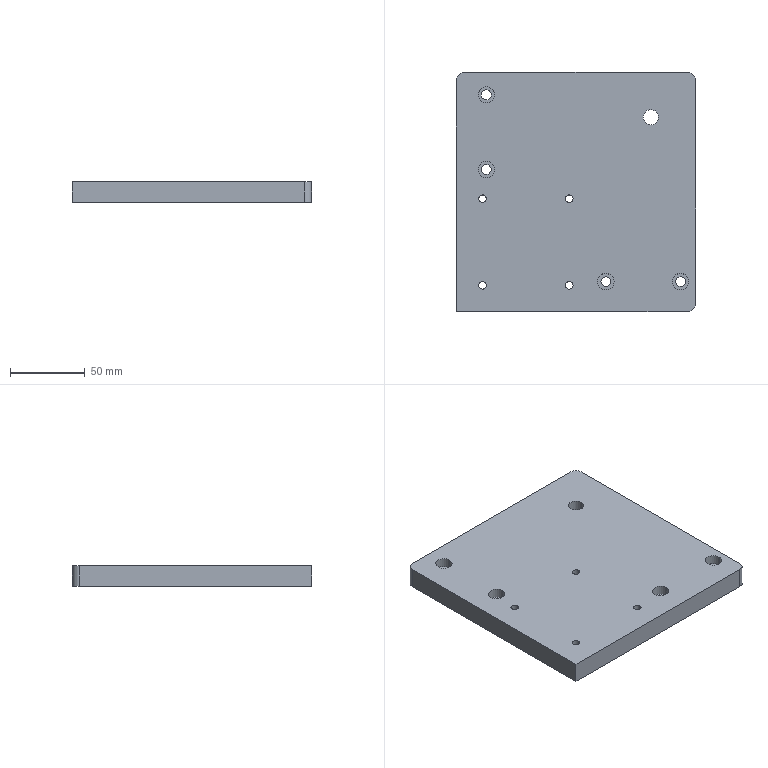Part | STEP file | HJ60 Fuma caster mounting plate -A0 | 1 solid | 39 faces | box 160 x 160 x 14 mm | volume 352458 mm3 | cylinder 29 | plane 10 | commonest cylinder face diameters 5 x8 6.6 x8 11 x8 10 x3 10.2 x2
STEP:
#1=CARTESIAN_POINT('',(-65.,-62.5,0.));
#2=VERTEX_POINT('',#1);
#3=CARTESIAN_POINT('',(-60.,-62.5,0.));
#4=VERTEX_POINT('',#3);
#5=CARTESIAN_POINT('',(-62.5,-62.5,0.));
#6=DIRECTION('',(0.,0.,1.));
#7=DIRECTION('',(1.,0.,0.));
#8=AXIS2_PLACEMENT_3D('',#5,#6,#7);
#9=CIRCLE('',#8,2.5);
#10=EDGE_CURVE('',#2,#4,#9,.T.);
#11=ORIENTED_EDGE('',*,*,#10,.F.);
#12=CARTESIAN_POINT('',(-65.,-62.5,14.));
#13=VERTEX_POINT('',#12);
#14=CARTESIAN_POINT('',(-65.,-62.5,14.));
#15=DIRECTION('',(0.,0.,1.));
#16=VECTOR('',#15,1000.);
#17=LINE('',#14,#16);
#18=EDGE_CURVE('',#2,#13,#17,.T.);
#19=ORIENTED_EDGE('',*,*,#18,.T.);
#20=CARTESIAN_POINT('',(-60.,-62.5,14.));
#21=VERTEX_POINT('',#20);
#22=CARTESIAN_POINT('',(-62.5,-62.5,14.));
#23=DIRECTION('',(0.,0.,-1.));
#24=DIRECTION('',(1.,0.,0.));
#25=AXIS2_PLACEMENT_3D('',#22,#23,#24);
#26=CIRCLE('',#25,2.5);
#27=EDGE_CURVE('',#21,#13,#26,.T.);
#28=ORIENTED_EDGE('',*,*,#27,.F.);
#29=CARTESIAN_POINT('',(-60.,-62.5,14.));
#30=DIRECTION('',(0.,0.,1.));
#31=VECTOR('',#30,1000.);
#32=LINE('',#29,#31);
#33=EDGE_CURVE('',#4,#21,#32,.T.);
#34=ORIENTED_EDGE('',*,*,#33,.F.);
#35=EDGE_LOOP('',(#11,#19,#28,#34));
#36=FACE_OUTER_BOUND('',#35,.T.);
#37=CARTESIAN_POINT('',(-62.5,-62.5,14.));
#38=DIRECTION('',(0.,0.,1.));
#39=DIRECTION('',(1.,0.,0.));
#40=AXIS2_PLACEMENT_3D('',#37,#38,#39);
#41=CYLINDRICAL_SURFACE('',#40,2.5);
#42=ADVANCED_FACE('',(#36),#41,.F.);
#43=CARTESIAN_POINT('',(-7.,-62.5,0.));
#44=VERTEX_POINT('',#43);
#45=CARTESIAN_POINT('',(-2.,-62.5,0.));
#46=VERTEX_POINT('',#45);
#47=CARTESIAN_POINT('',(-4.5,-62.5,0.));
#48=DIRECTION('',(0.,0.,1.));
#49=DIRECTION('',(1.,0.,0.));
#50=AXIS2_PLACEMENT_3D('',#47,#48,#49);
#51=CIRCLE('',#50,2.5);
#52=EDGE_CURVE('',#44,#46,#51,.T.);
#53=ORIENTED_EDGE('',*,*,#52,.F.);
#54=CARTESIAN_POINT('',(-7.,-62.5,14.));
#55=VERTEX_POINT('',#54);
#56=CARTESIAN_POINT('',(-7.,-62.5,14.));
#57=DIRECTION('',(0.,0.,1.));
#58=VECTOR('',#57,1000.);
#59=LINE('',#56,#58);
#60=EDGE_CURVE('',#44,#55,#59,.T.);
#61=ORIENTED_EDGE('',*,*,#60,.T.);
#62=CARTESIAN_POINT('',(-2.,-62.5,14.));
#63=VERTEX_POINT('',#62);
#64=CARTESIAN_POINT('',(-4.5,-62.5,14.));
#65=DIRECTION('',(0.,0.,-1.));
#66=DIRECTION('',(1.,0.,0.));
#67=AXIS2_PLACEMENT_3D('',#64,#65,#66);
#68=CIRCLE('',#67,2.5);
#69=EDGE_CURVE('',#63,#55,#68,.T.);
#70=ORIENTED_EDGE('',*,*,#69,.F.);
#71=CARTESIAN_POINT('',(-2.,-62.5,14.));
#72=DIRECTION('',(0.,0.,1.));
#73=VECTOR('',#72,1000.);
#74=LINE('',#71,#73);
#75=EDGE_CURVE('',#46,#63,#74,.T.);
#76=ORIENTED_EDGE('',*,*,#75,.F.);
#77=EDGE_LOOP('',(#53,#61,#70,#76));
#78=FACE_OUTER_BOUND('',#77,.T.);
#79=CARTESIAN_POINT('',(-4.5,-62.5,14.));
#80=DIRECTION('',(0.,0.,1.));
#81=DIRECTION('',(1.,0.,0.));
#82=AXIS2_PLACEMENT_3D('',#79,#80,#81);
#83=CYLINDRICAL_SURFACE('',#82,2.5);
#84=ADVANCED_FACE('',(#78),#83,.F.);
#85=CARTESIAN_POINT('',(-7.,-4.5,0.));
#86=VERTEX_POINT('',#85);
#87=CARTESIAN_POINT('',(-2.,-4.5,0.));
#88=VERTEX_POINT('',#87);
#89=CARTESIAN_POINT('',(-4.5,-4.5,0.));
#90=DIRECTION('',(0.,0.,1.));
#91=DIRECTION('',(1.,0.,0.));
#92=AXIS2_PLACEMENT_3D('',#89,#90,#91);
#93=CIRCLE('',#92,2.5);
#94=EDGE_CURVE('',#86,#88,#93,.T.);
#95=ORIENTED_EDGE('',*,*,#94,.F.);
#96=CARTESIAN_POINT('',(-7.,-4.5,14.));
#97=VERTEX_POINT('',#96);
#98=CARTESIAN_POINT('',(-7.,-4.5,14.));
#99=DIRECTION('',(0.,0.,1.));
#100=VECTOR('',#99,1000.);
#101=LINE('',#98,#100);
#102=EDGE_CURVE('',#86,#97,#101,.T.);
#103=ORIENTED_EDGE('',*,*,#102,.T.);
#104=CARTESIAN_POINT('',(-2.,-4.5,14.));
#105=VERTEX_POINT('',#104);
#106=CARTESIAN_POINT('',(-4.5,-4.5,14.));
#107=DIRECTION('',(0.,0.,-1.));
#108=DIRECTION('',(1.,0.,0.));
#109=AXIS2_PLACEMENT_3D('',#106,#107,#108);
#110=CIRCLE('',#109,2.5);
#111=EDGE_CURVE('',#105,#97,#110,.T.);
#112=ORIENTED_EDGE('',*,*,#111,.F.);
#113=CARTESIAN_POINT('',(-2.,-4.5,14.));
#114=DIRECTION('',(0.,0.,1.));
#115=VECTOR('',#114,1000.);
#116=LINE('',#113,#115);
#117=EDGE_CURVE('',#88,#105,#116,.T.);
#118=ORIENTED_EDGE('',*,*,#117,.F.);
#119=EDGE_LOOP('',(#95,#103,#112,#118));
#120=FACE_OUTER_BOUND('',#119,.T.);
#121=CARTESIAN_POINT('',(-4.5,-4.5,14.));
#122=DIRECTION('',(0.,0.,1.));
#123=DIRECTION('',(1.,0.,0.));
#124=AXIS2_PLACEMENT_3D('',#121,#122,#123);
#125=CYLINDRICAL_SURFACE('',#124,2.5);
#126=ADVANCED_FACE('',(#120),#125,.F.);
#127=CARTESIAN_POINT('',(-65.,-4.5,0.));
#128=VERTEX_POINT('',#127);
#129=CARTESIAN_POINT('',(-60.,-4.5,0.));
#130=VERTEX_POINT('',#129);
#131=CARTESIAN_POINT('',(-62.5,-4.5,0.));
#132=DIRECTION('',(0.,0.,1.));
#133=DIRECTION('',(1.,0.,0.));
#134=AXIS2_PLACEMENT_3D('',#131,#132,#133);
#135=CIRCLE('',#134,2.5);
#136=EDGE_CURVE('',#128,#130,#135,.T.);
#137=ORIENTED_EDGE('',*,*,#136,.F.);
#138=CARTESIAN_POINT('',(-65.,-4.5,14.));
#139=VERTEX_POINT('',#138);
#140=CARTESIAN_POINT('',(-65.,-4.5,14.));
#141=DIRECTION('',(0.,0.,1.));
#142=VECTOR('',#141,1000.);
#143=LINE('',#140,#142);
#144=EDGE_CURVE('',#128,#139,#143,.T.);
#145=ORIENTED_EDGE('',*,*,#144,.T.);
#146=CARTESIAN_POINT('',(-60.,-4.5,14.));
#147=VERTEX_POINT('',#146);
#148=CARTESIAN_POINT('',(-62.5,-4.5,14.));
#149=DIRECTION('',(0.,0.,-1.));
#150=DIRECTION('',(1.,0.,0.));
#151=AXIS2_PLACEMENT_3D('',#148,#149,#150);
#152=CIRCLE('',#151,2.5);
#153=EDGE_CURVE('',#147,#139,#152,.T.);
#154=ORIENTED_EDGE('',*,*,#153,.F.);
#155=CARTESIAN_POINT('',(-60.,-4.5,14.));
#156=DIRECTION('',(0.,0.,1.));
#157=VECTOR('',#156,1000.);
#158=LINE('',#155,#157);
#159=EDGE_CURVE('',#130,#147,#158,.T.);
#160=ORIENTED_EDGE('',*,*,#159,.F.);
#161=EDGE_LOOP('',(#137,#145,#154,#160));
#162=FACE_OUTER_BOUND('',#161,.T.);
#163=CARTESIAN_POINT('',(-62.5,-4.5,14.));
#164=DIRECTION('',(0.,0.,1.));
#165=DIRECTION('',(1.,0.,0.));
#166=AXIS2_PLACEMENT_3D('',#163,#164,#165);
#167=CYLINDRICAL_SURFACE('',#166,2.5);
#168=ADVANCED_FACE('',(#162),#167,.F.);
#169=CARTESIAN_POINT('',(44.9,50.,0.));
#170=VERTEX_POINT('',#169);
#171=CARTESIAN_POINT('',(55.1,50.,0.));
#172=VERTEX_POINT('',#171);
#173=CARTESIAN_POINT('',(50.,50.,0.));
#174=DIRECTION('',(0.,0.,1.));
#175=DIRECTION('',(1.,0.,0.));
#176=AXIS2_PLACEMENT_3D('',#173,#174,#175);
#177=CIRCLE('',#176,5.1);
#178=EDGE_CURVE('',#170,#172,#177,.T.);
#179=ORIENTED_EDGE('',*,*,#178,.F.);
#180=CARTESIAN_POINT('',(44.9,50.,14.));
#181=VERTEX_POINT('',#180);
#182=CARTESIAN_POINT('',(44.9,50.,14.));
#183=DIRECTION('',(0.,0.,1.));
#184=VECTOR('',#183,1000.);
#185=LINE('',#182,#184);
#186=EDGE_CURVE('',#170,#181,#185,.T.);
#187=ORIENTED_EDGE('',*,*,#186,.T.);
#188=CARTESIAN_POINT('',(55.1,50.,14.));
#189=VERTEX_POINT('',#188);
#190=CARTESIAN_POINT('',(50.,50.,14.));
#191=DIRECTION('',(0.,0.,-1.));
#192=DIRECTION('',(1.,0.,0.));
#193=AXIS2_PLACEMENT_3D('',#190,#191,#192);
#194=CIRCLE('',#193,5.1);
#195=EDGE_CURVE('',#189,#181,#194,.T.);
#196=ORIENTED_EDGE('',*,*,#195,.F.);
#197=CARTESIAN_POINT('',(55.1,50.,14.));
#198=DIRECTION('',(0.,0.,1.));
#199=VECTOR('',#198,1000.);
#200=LINE('',#197,#199);
#201=EDGE_CURVE('',#172,#189,#200,.T.);
#202=ORIENTED_EDGE('',*,*,#201,.F.);
#203=EDGE_LOOP('',(#179,#187,#196,#202));
#204=FACE_OUTER_BOUND('',#203,.T.);
#205=CARTESIAN_POINT('',(50.,50.,14.));
#206=DIRECTION('',(0.,0.,1.));
#207=DIRECTION('',(1.,0.,0.));
#208=AXIS2_PLACEMENT_3D('',#205,#206,#207);
#209=CYLINDRICAL_SURFACE('',#208,5.1);
#210=ADVANCED_FACE('',(#204),#209,.F.);
#211=CARTESIAN_POINT('',(16.7,-60.,0.));
#212=VERTEX_POINT('',#211);
#213=CARTESIAN_POINT('',(23.3,-60.,0.));
#214=VERTEX_POINT('',#213);
#215=CARTESIAN_POINT('',(20.,-60.,0.));
#216=DIRECTION('',(0.,0.,1.));
#217=DIRECTION('',(1.,0.,0.));
#218=AXIS2_PLACEMENT_3D('',#215,#216,#217);
#219=CIRCLE('',#218,3.3);
#220=EDGE_CURVE('',#212,#214,#219,.T.);
#221=ORIENTED_EDGE('',*,*,#220,.F.);
#222=CARTESIAN_POINT('',(16.7,-60.,7.6));
#223=VERTEX_POINT('',#222);
#224=CARTESIAN_POINT('',(16.7,-60.,14.));
#225=DIRECTION('',(0.,0.,1.));
#226=VECTOR('',#225,1000.);
#227=LINE('',#224,#226);
#228=EDGE_CURVE('',#212,#223,#227,.T.);
#229=ORIENTED_EDGE('',*,*,#228,.T.);
#230=CARTESIAN_POINT('',(23.3,-60.,7.6));
#231=VERTEX_POINT('',#230);
#232=CARTESIAN_POINT('',(20.,-60.,7.6));
#233=DIRECTION('',(0.,0.,-1.));
#234=DIRECTION('',(1.,0.,0.));
#235=AXIS2_PLACEMENT_3D('',#232,#233,#234);
#236=CIRCLE('',#235,3.3);
#237=EDGE_CURVE('',#231,#223,#236,.T.);
#238=ORIENTED_EDGE('',*,*,#237,.F.);
#239=CARTESIAN_POINT('',(23.3,-60.,14.));
#240=DIRECTION('',(0.,0.,1.));
#241=VECTOR('',#240,1000.);
#242=LINE('',#239,#241);
#243=EDGE_CURVE('',#214,#231,#242,.T.);
#244=ORIENTED_EDGE('',*,*,#243,.F.);
#245=EDGE_LOOP('',(#221,#229,#238,#244));
#246=FACE_OUTER_BOUND('',#245,.T.);
#247=CARTESIAN_POINT('',(20.,-60.,14.));
#248=DIRECTION('',(0.,0.,1.));
#249=DIRECTION('',(1.,0.,0.));
#250=AXIS2_PLACEMENT_3D('',#247,#248,#249);
#251=CYLINDRICAL_SURFACE('',#250,3.3);
#252=ADVANCED_FACE('',(#246),#251,.F.);
#253=CARTESIAN_POINT('',(66.7,-60.,0.));
#254=VERTEX_POINT('',#253);
#255=CARTESIAN_POINT('',(73.3,-60.,0.));
#256=VERTEX_POINT('',#255);
#257=CARTESIAN_POINT('',(70.,-60.,0.));
#258=DIRECTION('',(0.,0.,1.));
#259=DIRECTION('',(1.,0.,0.));
#260=AXIS2_PLACEMENT_3D('',#257,#258,#259);
#261=CIRCLE('',#260,3.3);
#262=EDGE_CURVE('',#254,#256,#261,.T.);
#263=ORIENTED_EDGE('',*,*,#262,.F.);
#264=CARTESIAN_POINT('',(66.7,-60.,7.6));
#265=VERTEX_POINT('',#264);
#266=CARTESIAN_POINT('',(66.7,-60.,14.));
#267=DIRECTION('',(0.,0.,1.));
#268=VECTOR('',#267,1000.);
#269=LINE('',#266,#268);
#270=EDGE_CURVE('',#254,#265,#269,.T.);
#271=ORIENTED_EDGE('',*,*,#270,.T.);
#272=CARTESIAN_POINT('',(73.3,-60.,7.6));
#273=VERTEX_POINT('',#272);
#274=CARTESIAN_POINT('',(70.,-60.,7.6));
#275=DIRECTION('',(0.,0.,-1.));
#276=DIRECTION('',(1.,0.,0.));
#277=AXIS2_PLACEMENT_3D('',#274,#275,#276);
#278=CIRCLE('',#277,3.3);
#279=EDGE_CURVE('',#273,#265,#278,.T.);
#280=ORIENTED_EDGE('',*,*,#279,.F.);
#281=CARTESIAN_POINT('',(73.3,-60.,14.));
#282=DIRECTION('',(0.,0.,1.));
#283=VECTOR('',#282,1000.);
#284=LINE('',#281,#283);
#285=EDGE_CURVE('',#256,#273,#284,.T.);
#286=ORIENTED_EDGE('',*,*,#285,.F.);
#287=EDGE_LOOP('',(#263,#271,#280,#286));
#288=FACE_OUTER_BOUND('',#287,.T.);
#289=CARTESIAN_POINT('',(70.,-60.,14.));
#290=DIRECTION('',(0.,0.,1.));
#291=DIRECTION('',(1.,0.,0.));
#292=AXIS2_PLACEMENT_3D('',#289,#290,#291);
#293=CYLINDRICAL_SURFACE('',#292,3.3);
#294=ADVANCED_FACE('',(#288),#293,.F.);
#295=CARTESIAN_POINT('',(-63.3,15.,0.));
#296=VERTEX_POINT('',#295);
#297=CARTESIAN_POINT('',(-56.7,15.,0.));
#298=VERTEX_POINT('',#297);
#299=CARTESIAN_POINT('',(-60.,15.,0.));
#300=DIRECTION('',(0.,0.,1.));
#301=DIRECTION('',(1.,0.,0.));
#302=AXIS2_PLACEMENT_3D('',#299,#300,#301);
#303=CIRCLE('',#302,3.3);
#304=EDGE_CURVE('',#296,#298,#303,.T.);
#305=ORIENTED_EDGE('',*,*,#304,.F.);
#306=CARTESIAN_POINT('',(-63.3,15.,7.6));
#307=VERTEX_POINT('',#306);
#308=CARTESIAN_POINT('',(-63.3,15.,14.));
#309=DIRECTION('',(0.,0.,1.));
#310=VECTOR('',#309,1000.);
#311=LINE('',#308,#310);
#312=EDGE_CURVE('',#296,#307,#311,.T.);
#313=ORIENTED_EDGE('',*,*,#312,.T.);
#314=CARTESIAN_POINT('',(-56.7,15.,7.6));
#315=VERTEX_POINT('',#314);
#316=CARTESIAN_POINT('',(-60.,15.,7.6));
#317=DIRECTION('',(0.,0.,-1.));
#318=DIRECTION('',(1.,0.,0.));
#319=AXIS2_PLACEMENT_3D('',#316,#317,#318);
#320=CIRCLE('',#319,3.3);
#321=EDGE_CURVE('',#315,#307,#320,.T.);
#322=ORIENTED_EDGE('',*,*,#321,.F.);
#323=CARTESIAN_POINT('',(-56.7,15.,14.));
#324=DIRECTION('',(0.,0.,1.));
#325=VECTOR('',#324,1000.);
#326=LINE('',#323,#325);
#327=EDGE_CURVE('',#298,#315,#326,.T.);
#328=ORIENTED_EDGE('',*,*,#327,.F.);
#329=EDGE_LOOP('',(#305,#313,#322,#328));
#330=FACE_OUTER_BOUND('',#329,.T.);
#331=CARTESIAN_POINT('',(-60.,15.,14.));
#332=DIRECTION('',(0.,0.,1.));
#333=DIRECTION('',(1.,0.,0.));
#334=AXIS2_PLACEMENT_3D('',#331,#332,#333);
#335=CYLINDRICAL_SURFACE('',#334,3.3);
#336=ADVANCED_FACE('',(#330),#335,.F.);
#337=CARTESIAN_POINT('',(-63.3,65.,0.));
#338=VERTEX_POINT('',#337);
#339=CARTESIAN_POINT('',(-56.7,65.,0.));
#340=VERTEX_POINT('',#339);
#341=CARTESIAN_POINT('',(-60.,65.,0.));
#342=DIRECTION('',(0.,0.,1.));
#343=DIRECTION('',(1.,0.,0.));
#344=AXIS2_PLACEMENT_3D('',#341,#342,#343);
#345=CIRCLE('',#344,3.3);
#346=EDGE_CURVE('',#338,#340,#345,.T.);
#347=ORIENTED_EDGE('',*,*,#346,.F.);
#348=CARTESIAN_POINT('',(-63.3,65.,7.6));
#349=VERTEX_POINT('',#348);
#350=CARTESIAN_POINT('',(-63.3,65.,14.));
#351=DIRECTION('',(0.,0.,1.));
#352=VECTOR('',#351,1000.);
#353=LINE('',#350,#352);
#354=EDGE_CURVE('',#338,#349,#353,.T.);
#355=ORIENTED_EDGE('',*,*,#354,.T.);
#356=CARTESIAN_POINT('',(-56.7,65.,7.6));
#357=VERTEX_POINT('',#356);
#358=CARTESIAN_POINT('',(-60.,65.,7.6));
#359=DIRECTION('',(0.,0.,-1.));
#360=DIRECTION('',(1.,0.,0.));
#361=AXIS2_PLACEMENT_3D('',#358,#359,#360);
#362=CIRCLE('',#361,3.3);
#363=EDGE_CURVE('',#357,#349,#362,.T.);
#364=ORIENTED_EDGE('',*,*,#363,.F.);
#365=CARTESIAN_POINT('',(-56.7,65.,14.));
#366=DIRECTION('',(0.,0.,1.));
#367=VECTOR('',#366,1000.);
#368=LINE('',#365,#367);
#369=EDGE_CURVE('',#340,#357,#368,.T.);
#370=ORIENTED_EDGE('',*,*,#369,.F.);
#371=EDGE_LOOP('',(#347,#355,#364,#370));
#372=FACE_OUTER_BOUND('',#371,.T.);
#373=CARTESIAN_POINT('',(-60.,65.,14.));
#374=DIRECTION('',(0.,0.,1.));
#375=DIRECTION('',(1.,0.,0.));
#376=AXIS2_PLACEMENT_3D('',#373,#374,#375);
#377=CYLINDRICAL_SURFACE('',#376,3.3);
#378=ADVANCED_FACE('',(#372),#377,.F.);
#379=CARTESIAN_POINT('',(25.5,-60.,7.6));
#380=VERTEX_POINT('',#379);
#381=CARTESIAN_POINT('',(14.5,-60.,7.6));
#382=VERTEX_POINT('',#381);
#383=CARTESIAN_POINT('',(20.,-60.,7.6));
#384=DIRECTION('',(0.,0.,-1.));
#385=DIRECTION('',(1.,0.,0.));
#386=AXIS2_PLACEMENT_3D('',#383,#384,#385);
#387=CIRCLE('',#386,5.5);
#388=EDGE_CURVE('',#380,#382,#387,.T.);
#389=ORIENTED_EDGE('',*,*,#388,.T.);
#390=CARTESIAN_POINT('',(14.5,-60.,14.));
#391=VERTEX_POINT('',#390);
#392=CARTESIAN_POINT('',(14.5,-60.,14.));
#393=DIRECTION('',(0.,0.,1.));
#394=VECTOR('',#393,1000.);
#395=LINE('',#392,#394);
#396=EDGE_CURVE('',#382,#391,#395,.T.);
#397=ORIENTED_EDGE('',*,*,#396,.T.);
#398=CARTESIAN_POINT('',(25.5,-60.,14.));
#399=VERTEX_POINT('',#398);
#400=CARTESIAN_POINT('',(20.,-60.,14.));
#401=DIRECTION('',(0.,0.,1.));
#402=DIRECTION('',(1.,0.,0.));
#403=AXIS2_PLACEMENT_3D('',#400,#401,#402);
#404=CIRCLE('',#403,5.5);
#405=EDGE_CURVE('',#391,#399,#404,.T.);
#406=ORIENTED_EDGE('',*,*,#405,.T.);
#407=CARTESIAN_POINT('',(25.5,-60.,14.));
#408=DIRECTION('',(0.,0.,1.));
#409=VECTOR('',#408,1000.);
#410=LINE('',#407,#409);
#411=EDGE_CURVE('',#380,#399,#410,.T.);
#412=ORIENTED_EDGE('',*,*,#411,.F.);
#413=EDGE_LOOP('',(#389,#397,#406,#412));
#414=FACE_OUTER_BOUND('',#413,.T.);
#415=CARTESIAN_POINT('',(20.,-60.,14.));
#416=DIRECTION('',(0.,0.,1.));
#417=DIRECTION('',(1.,0.,0.));
#418=AXIS2_PLACEMENT_3D('',#415,#416,#417);
#419=CYLINDRICAL_SURFACE('',#418,5.5);
#420=ADVANCED_FACE('',(#414),#419,.F.);
#421=CARTESIAN_POINT('',(75.5,-60.,7.6));
#422=VERTEX_POINT('',#421);
#423=CARTESIAN_POINT('',(64.5,-60.,7.6));
#424=VERTEX_POINT('',#423);
#425=CARTESIAN_POINT('',(70.,-60.,7.6));
#426=DIRECTION('',(0.,0.,-1.));
#427=DIRECTION('',(1.,0.,0.));
#428=AXIS2_PLACEMENT_3D('',#425,#426,#427);
#429=CIRCLE('',#428,5.5);
#430=EDGE_CURVE('',#422,#424,#429,.T.);
#431=ORIENTED_EDGE('',*,*,#430,.T.);
#432=CARTESIAN_POINT('',(64.5,-60.,14.));
#433=VERTEX_POINT('',#432);
#434=CARTESIAN_POINT('',(64.5,-60.,14.));
#435=DIRECTION('',(0.,0.,1.));
#436=VECTOR('',#435,1000.);
#437=LINE('',#434,#436);
#438=EDGE_CURVE('',#424,#433,#437,.T.);
#439=ORIENTED_EDGE('',*,*,#438,.T.);
#440=CARTESIAN_POINT('',(75.5,-60.,14.));
#441=VERTEX_POINT('',#440);
#442=CARTESIAN_POINT('',(70.,-60.,14.));
#443=DIRECTION('',(0.,0.,1.));
#444=DIRECTION('',(1.,0.,0.));
#445=AXIS2_PLACEMENT_3D('',#442,#443,#444);
#446=CIRCLE('',#445,5.5);
#447=EDGE_CURVE('',#433,#441,#446,.T.);
#448=ORIENTED_EDGE('',*,*,#447,.T.);
#449=CARTESIAN_POINT('',(75.5,-60.,14.));
#450=DIRECTION('',(0.,0.,1.));
#451=VECTOR('',#450,1000.);
#452=LINE('',#449,#451);
#453=EDGE_CURVE('',#422,#441,#452,.T.);
#454=ORIENTED_EDGE('',*,*,#453,.F.);
#455=EDGE_LOOP('',(#431,#439,#448,#454));
#456=FACE_OUTER_BOUND('',#455,.T.);
#457=CARTESIAN_POINT('',(70.,-60.,14.));
#458=DIRECTION('',(0.,0.,1.));
#459=DIRECTION('',(1.,0.,0.));
#460=AXIS2_PLACEMENT_3D('',#457,#458,#459);
#461=CYLINDRICAL_SURFACE('',#460,5.5);
#462=ADVANCED_FACE('',(#456),#461,.F.);
#463=CARTESIAN_POINT('',(-54.5,15.,7.6));
#464=VERTEX_POINT('',#463);
#465=CARTESIAN_POINT('',(-65.5,15.,7.6));
#466=VERTEX_POINT('',#465);
#467=CARTESIAN_POINT('',(-60.,15.,7.6));
#468=DIRECTION('',(0.,0.,-1.));
#469=DIRECTION('',(1.,0.,0.));
#470=AXIS2_PLACEMENT_3D('',#467,#468,#469);
#471=CIRCLE('',#470,5.5);
#472=EDGE_CURVE('',#464,#466,#471,.T.);
#473=ORIENTED_EDGE('',*,*,#472,.T.);
#474=CARTESIAN_POINT('',(-65.5,15.,14.));
#475=VERTEX_POINT('',#474);
#476=CARTESIAN_POINT('',(-65.5,15.,14.));
#477=DIRECTION('',(0.,0.,1.));
#478=VECTOR('',#477,1000.);
#479=LINE('',#476,#478);
#480=EDGE_CURVE('',#466,#475,#479,.T.);
#481=ORIENTED_EDGE('',*,*,#480,.T.);
#482=CARTESIAN_POINT('',(-54.5,15.,14.));
#483=VERTEX_POINT('',#482);
#484=CARTESIAN_POINT('',(-60.,15.,14.));
#485=DIRECTION('',(0.,0.,1.));
#486=DIRECTION('',(1.,0.,0.));
#487=AXIS2_PLACEMENT_3D('',#484,#485,#486);
#488=CIRCLE('',#487,5.5);
#489=EDGE_CURVE('',#475,#483,#488,.T.);
#490=ORIENTED_EDGE('',*,*,#489,.T.);
#491=CARTESIAN_POINT('',(-54.5,15.,14.));
#492=DIRECTION('',(0.,0.,1.));
#493=VECTOR('',#492,1000.);
#494=LINE('',#491,#493);
#495=EDGE_CURVE('',#464,#483,#494,.T.);
#496=ORIENTED_EDGE('',*,*,#495,.F.);
#497=EDGE_LOOP('',(#473,#481,#490,#496));
#498=FACE_OUTER_BOUND('',#497,.T.);
#499=CARTESIAN_POINT('',(-60.,15.,14.));
#500=DIRECTION('',(0.,0.,1.));
#501=DIRECTION('',(1.,0.,0.));
#502=AXIS2_PLACEMENT_3D('',#499,#500,#501);
#503=CYLINDRICAL_SURFACE('',#502,5.5);
#504=ADVANCED_FACE('',(#498),#503,.F.);
#505=CARTESIAN_POINT('',(-54.5,65.,7.6));
#506=VERTEX_POINT('',#505);
#507=CARTESIAN_POINT('',(-65.5,65.,7.6));
#508=VERTEX_POINT('',#507);
#509=CARTESIAN_POINT('',(-60.,65.,7.6));
#510=DIRECTION('',(0.,0.,-1.));
#511=DIRECTION('',(1.,0.,0.));
#512=AXIS2_PLACEMENT_3D('',#509,#510,#511);
#513=CIRCLE('',#512,5.5);
#514=EDGE_CURVE('',#506,#508,#513,.T.);
#515=ORIENTED_EDGE('',*,*,#514,.T.);
#516=CARTESIAN_POINT('',(-65.5,65.,14.));
#517=VERTEX_POINT('',#516);
#518=CARTESIAN_POINT('',(-65.5,65.,14.));
#519=DIRECTION('',(0.,0.,1.));
#520=VECTOR('',#519,1000.);
#521=LINE('',#518,#520);
#522=EDGE_CURVE('',#508,#517,#521,.T.);
#523=ORIENTED_EDGE('',*,*,#522,.T.);
#524=CARTESIAN_POINT('',(-54.5,65.,14.));
#525=VERTEX_POINT('',#524);
#526=CARTESIAN_POINT('',(-60.,65.,14.));
#527=DIRECTION('',(0.,0.,1.));
#528=DIRECTION('',(1.,0.,0.));
#529=AXIS2_PLACEMENT_3D('',#526,#527,#528);
#530=CIRCLE('',#529,5.5);
#531=EDGE_CURVE('',#517,#525,#530,.T.);
#532=ORIENTED_EDGE('',*,*,#531,.T.);
#533=CARTESIAN_POINT('',(-54.5,65.,14.));
#534=DIRECTION('',(0.,0.,1.));
#535=VECTOR('',#534,1000.);
#536=LINE('',#533,#535);
#537=EDGE_CURVE('',#506,#525,#536,.T.);
#538=ORIENTED_EDGE('',*,*,#537,.F.);
#539=EDGE_LOOP('',(#515,#523,#532,#538));
#540=FACE_OUTER_BOUND('',#539,.T.);
#541=CARTESIAN_POINT('',(-60.,65.,14.));
#542=DIRECTION('',(0.,0.,1.));
#543=DIRECTION('',(1.,0.,0.));
#544=AXIS2_PLACEMENT_3D('',#541,#542,#543);
#545=CYLINDRICAL_SURFACE('',#544,5.5);
#546=ADVANCED_FACE('',(#540),#545,.F.);
#547=CARTESIAN_POINT('',(80.,75.,0.));
#548=VERTEX_POINT('',#547);
#549=CARTESIAN_POINT('',(80.,-75.,0.));
#550=VERTEX_POINT('',#549);
#551=CARTESIAN_POINT('',(80.,-75.,0.));
#552=DIRECTION('',(0.,-1.,0.));
#553=VECTOR('',#552,1000.);
#554=LINE('',#551,#553);
#555=EDGE_CURVE('',#548,#550,#554,.T.);
#556=ORIENTED_EDGE('',*,*,#555,.T.);
#557=CARTESIAN_POINT('',(75.,-80.,0.));
#558=VERTEX_POINT('',#557);
#559=CARTESIAN_POINT('',(75.,-75.,0.));
#560=DIRECTION('',(0.,0.,-1.));
#561=DIRECTION('',(-1.,0.,0.));
#562=AXIS2_PLACEMENT_3D('',#559,#560,#561);
#563=CIRCLE('',#562,5.);
#564=EDGE_CURVE('',#550,#558,#563,.T.);
#565=ORIENTED_EDGE('',*,*,#564,.T.);
#566=CARTESIAN_POINT('',(-80.,-80.,0.));
#567=VERTEX_POINT('',#566);
#568=CARTESIAN_POINT('',(75.,-80.,0.));
#569=DIRECTION('',(-1.,0.,0.));
#570=VECTOR('',#569,1000.);
#571=LINE('',#568,#570);
#572=EDGE_CURVE('',#558,#567,#571,.T.);
#573=ORIENTED_EDGE('',*,*,#572,.T.);
#574=CARTESIAN_POINT('',(-80.,75.,0.));
#575=VERTEX_POINT('',#574);
#576=CARTESIAN_POINT('',(-80.,-75.,0.));
#577=DIRECTION('',(0.,1.,0.));
#578=VECTOR('',#577,1000.);
#579=LINE('',#576,#578);
#580=EDGE_CURVE('',#567,#575,#579,.T.);
#581=ORIENTED_EDGE('',*,*,#580,.T.);
#582=CARTESIAN_POINT('',(-75.,80.,0.));
#583=VERTEX_POINT('',#582);
#584=CARTESIAN_POINT('',(-75.,75.,0.));
#585=DIRECTION('',(0.,0.,-1.));
#586=DIRECTION('',(-1.,0.,0.));
#587=AXIS2_PLACEMENT_3D('',#584,#585,#586);
#588=CIRCLE('',#587,5.);
#589=EDGE_CURVE('',#575,#583,#588,.T.);
#590=ORIENTED_EDGE('',*,*,#589,.T.);
#591=CARTESIAN_POINT('',(75.,80.,0.));
#592=VERTEX_POINT('',#591);
#593=CARTESIAN_POINT('',(75.,80.,0.));
#594=DIRECTION('',(1.,0.,0.));
#595=VECTOR('',#594,1000.);
#596=LINE('',#593,#595);
#597=EDGE_CURVE('',#583,#592,#596,.T.);
#598=ORIENTED_EDGE('',*,*,#597,.T.);
#599=CARTESIAN_POINT('',(75.,75.,0.));
#600=DIRECTION('',(0.,0.,-1.));
#601=DIRECTION('',(-1.,0.,0.));
#602=AXIS2_PLACEMENT_3D('',#599,#600,#601);
#603=CIRCLE('',#602,5.);
#604=EDGE_CURVE('',#592,#548,#603,.T.);
#605=ORIENTED_EDGE('',*,*,#604,.T.);
#606=EDGE_LOOP('',(#556,#565,#573,#581,#590,#598,#605));
#607=FACE_OUTER_BOUND('',#606,.T.);
#608=CARTESIAN_POINT('',(-62.5,-62.5,0.));
#609=DIRECTION('',(0.,0.,1.));
#610=DIRECTION('',(1.,0.,0.));
#611=AXIS2_PLACEMENT_3D('',#608,#609,#610);
#612=CIRCLE('',#611,2.5);
#613=EDGE_CURVE('',#4,#2,#612,.T.);
#614=ORIENTED_EDGE('',*,*,#613,.T.);
#615=ORIENTED_EDGE('',*,*,#10,.T.);
#616=EDGE_LOOP('',(#614,#615));
#617=FACE_BOUND('',#616,.T.);
#618=CARTESIAN_POINT('',(-4.5,-62.5,0.));
#619=DIRECTION('',(0.,0.,1.));
#620=DIRECTION('',(1.,0.,0.));
#621=AXIS2_PLACEMENT_3D('',#618,#619,#620);
#622=CIRCLE('',#621,2.5);
#623=EDGE_CURVE('',#46,#44,#622,.T.);
#624=ORIENTED_EDGE('',*,*,#623,.T.);
#625=ORIENTED_EDGE('',*,*,#52,.T.);
#626=EDGE_LOOP('',(#624,#625));
#627=FACE_BOUND('',#626,.T.);
#628=CARTESIAN_POINT('',(-4.5,-4.5,0.));
#629=DIRECTION('',(0.,0.,1.));
#630=DIRECTION('',(1.,0.,0.));
#631=AXIS2_PLACEMENT_3D('',#628,#629,#630);
#632=CIRCLE('',#631,2.5);
#633=EDGE_CURVE('',#88,#86,#632,.T.);
#634=ORIENTED_EDGE('',*,*,#633,.T.);
#635=ORIENTED_EDGE('',*,*,#94,.T.);
#636=EDGE_LOOP('',(#634,#635));
#637=FACE_BOUND('',#636,.T.);
#638=CARTESIAN_POINT('',(-62.5,-4.5,0.));
#639=DIRECTION('',(0.,0.,1.));
#640=DIRECTION('',(1.,0.,0.));
#641=AXIS2_PLACEMENT_3D('',#638,#639,#640);
#642=CIRCLE('',#641,2.5);
#643=EDGE_CURVE('',#130,#128,#642,.T.);
#644=ORIENTED_EDGE('',*,*,#643,.T.);
#645=ORIENTED_EDGE('',*,*,#136,.T.);
#646=EDGE_LOOP('',(#644,#645));
#647=FACE_BOUND('',#646,.T.);
#648=CARTESIAN_POINT('',(50.,50.,0.));
#649=DIRECTION('',(0.,0.,1.));
#650=DIRECTION('',(1.,0.,0.));
#651=AXIS2_PLACEMENT_3D('',#648,#649,#650);
#652=CIRCLE('',#651,5.1);
#653=EDGE_CURVE('',#172,#170,#652,.T.);
#654=ORIENTED_EDGE('',*,*,#653,.T.);
#655=ORIENTED_EDGE('',*,*,#178,.T.);
#656=EDGE_LOOP('',(#654,#655));
#657=FACE_BOUND('',#656,.T.);
#658=CARTESIAN_POINT('',(20.,-60.,0.));
#659=DIRECTION('',(0.,0.,1.));
#660=DIRECTION('',(1.,0.,0.));
#661=AXIS2_PLACEMENT_3D('',#658,#659,#660);
#662=CIRCLE('',#661,3.3);
#663=EDGE_CURVE('',#214,#212,#662,.T.);
#664=ORIENTED_EDGE('',*,*,#663,.T.);
#665=ORIENTED_EDGE('',*,*,#220,.T.);
#666=EDGE_LOOP('',(#664,#665));
#667=FACE_BOUND('',#666,.T.);
#668=CARTESIAN_POINT('',(70.,-60.,0.));
#669=DIRECTION('',(0.,0.,1.));
#670=DIRECTION('',(1.,0.,0.));
#671=AXIS2_PLACEMENT_3D('',#668,#669,#670);
#672=CIRCLE('',#671,3.3);
#673=EDGE_CURVE('',#256,#254,#672,.T.);
#674=ORIENTED_EDGE('',*,*,#673,.T.);
#675=ORIENTED_EDGE('',*,*,#262,.T.);
#676=EDGE_LOOP('',(#674,#675));
#677=FACE_BOUND('',#676,.T.);
#678=CARTESIAN_POINT('',(-60.,15.,0.));
#679=DIRECTION('',(0.,0.,1.));
#680=DIRECTION('',(1.,0.,0.));
#681=AXIS2_PLACEMENT_3D('',#678,#679,#680);
#682=CIRCLE('',#681,3.3);
#683=EDGE_CURVE('',#298,#296,#682,.T.);
#684=ORIENTED_EDGE('',*,*,#683,.T.);
#685=ORIENTED_EDGE('',*,*,#304,.T.);
#686=EDGE_LOOP('',(#684,#685));
#687=FACE_BOUND('',#686,.T.);
#688=CARTESIAN_POINT('',(-60.,65.,0.));
#689=DIRECTION('',(0.,0.,1.));
#690=DIRECTION('',(1.,0.,0.));
#691=AXIS2_PLACEMENT_3D('',#688,#689,#690);
#692=CIRCLE('',#691,3.3);
#693=EDGE_CURVE('',#340,#338,#692,.T.);
#694=ORIENTED_EDGE('',*,*,#693,.T.);
#695=ORIENTED_EDGE('',*,*,#346,.T.);
#696=EDGE_LOOP('',(#694,#695));
#697=FACE_BOUND('',#696,.T.);
#698=CARTESIAN_POINT('',(75.,-75.,0.));
#699=DIRECTION('',(0.,0.,-1.));
#700=DIRECTION('',(-1.,0.,0.));
#701=AXIS2_PLACEMENT_3D('',#698,#699,#700);
#702=PLANE('',#701);
#703=ADVANCED_FACE('',(#607,#617,#627,#637,#647,#657,#667,#677,#687,#697),#702,.T.);
#704=CARTESIAN_POINT('',(80.,-75.,14.));
#705=VERTEX_POINT('',#704);
#706=CARTESIAN_POINT('',(75.,-80.,14.));
#707=VERTEX_POINT('',#706);
#708=CARTESIAN_POINT('',(75.,-75.,14.));
#709=DIRECTION('',(0.,0.,-1.));
#710=DIRECTION('',(-1.,0.,0.));
#711=AXIS2_PLACEMENT_3D('',#708,#709,#710);
#712=CIRCLE('',#711,5.);
#713=EDGE_CURVE('',#705,#707,#712,.T.);
#714=ORIENTED_EDGE('',*,*,#713,.T.);
#715=CARTESIAN_POINT('',(75.,-80.,14.));
#716=DIRECTION('',(0.,0.,-1.));
#717=VECTOR('',#716,1000.);
#718=LINE('',#715,#717);
#719=EDGE_CURVE('',#707,#558,#718,.T.);
#720=ORIENTED_EDGE('',*,*,#719,.T.);
#721=ORIENTED_EDGE('',*,*,#564,.F.);
#722=CARTESIAN_POINT('',(80.,-75.,14.));
#723=DIRECTION('',(0.,0.,1.));
#724=VECTOR('',#723,1000.);
#725=LINE('',#722,#724);
#726=EDGE_CURVE('',#550,#705,#725,.T.);
#727=ORIENTED_EDGE('',*,*,#726,.T.);
#728=EDGE_LOOP('',(#714,#720,#721,#727));
#729=FACE_OUTER_BOUND('',#728,.T.);
#730=CARTESIAN_POINT('',(75.,-75.,14.));
#731=DIRECTION('',(0.,0.,-1.));
#732=DIRECTION('',(-1.,0.,0.));
#733=AXIS2_PLACEMENT_3D('',#730,#731,#732);
#734=CYLINDRICAL_SURFACE('',#733,5.);
#735=ADVANCED_FACE('',(#729),#734,.T.);
#736=CARTESIAN_POINT('',(80.,75.,14.));
#737=VERTEX_POINT('',#736);
#738=CARTESIAN_POINT('',(80.,75.,14.));
#739=DIRECTION('',(0.,0.,-1.));
#740=VECTOR('',#739,1000.);
#741=LINE('',#738,#740);
#742=EDGE_CURVE('',#737,#548,#741,.T.);
#743=ORIENTED_EDGE('',*,*,#742,.F.);
#744=CARTESIAN_POINT('',(80.,-75.,14.));
#745=DIRECTION('',(0.,1.,0.));
#746=VECTOR('',#745,1000.);
#747=LINE('',#744,#746);
#748=EDGE_CURVE('',#705,#737,#747,.T.);
#749=ORIENTED_EDGE('',*,*,#748,.F.);
#750=ORIENTED_EDGE('',*,*,#726,.F.);
#751=ORIENTED_EDGE('',*,*,#555,.F.);
#752=EDGE_LOOP('',(#743,#749,#750,#751));
#753=FACE_OUTER_BOUND('',#752,.T.);
#754=CARTESIAN_POINT('',(80.,-75.,14.));
#755=DIRECTION('',(-1.,0.,0.));
#756=DIRECTION('',(0.,0.,1.));
#757=AXIS2_PLACEMENT_3D('',#754,#755,#756);
#758=PLANE('',#757);
#759=ADVANCED_FACE('',(#753),#758,.F.);
#760=CARTESIAN_POINT('',(75.,80.,14.));
#761=VERTEX_POINT('',#760);
#762=CARTESIAN_POINT('',(75.,75.,14.));
#763=DIRECTION('',(0.,0.,-1.));
#764=DIRECTION('',(-1.,0.,0.));
#765=AXIS2_PLACEMENT_3D('',#762,#763,#764);
#766=CIRCLE('',#765,5.);
#767=EDGE_CURVE('',#761,#737,#766,.T.);
#768=ORIENTED_EDGE('',*,*,#767,.T.);
#769=ORIENTED_EDGE('',*,*,#742,.T.);
#770=ORIENTED_EDGE('',*,*,#604,.F.);
#771=CARTESIAN_POINT('',(75.,80.,14.));
#772=DIRECTION('',(0.,0.,1.));
#773=VECTOR('',#772,1000.);
#774=LINE('',#771,#773);
#775=EDGE_CURVE('',#592,#761,#774,.T.);
#776=ORIENTED_EDGE('',*,*,#775,.T.);
#777=EDGE_LOOP('',(#768,#769,#770,#776));
#778=FACE_OUTER_BOUND('',#777,.T.);
#779=CARTESIAN_POINT('',(75.,75.,14.));
#780=DIRECTION('',(0.,0.,-1.));
#781=DIRECTION('',(-1.,0.,0.));
#782=AXIS2_PLACEMENT_3D('',#779,#780,#781);
#783=CYLINDRICAL_SURFACE('',#782,5.);
#784=ADVANCED_FACE('',(#778),#783,.T.);
#785=CARTESIAN_POINT('',(-75.,80.,14.));
#786=VERTEX_POINT('',#785);
#787=CARTESIAN_POINT('',(-75.,80.,14.));
#788=DIRECTION('',(0.,0.,-1.));
#789=VECTOR('',#788,1000.);
#790=LINE('',#787,#789);
#791=EDGE_CURVE('',#786,#583,#790,.T.);
#792=ORIENTED_EDGE('',*,*,#791,.F.);
#793=CARTESIAN_POINT('',(-75.,80.,14.));
#794=DIRECTION('',(-1.,0.,0.));
#795=VECTOR('',#794,1000.);
#796=LINE('',#793,#795);
#797=EDGE_CURVE('',#761,#786,#796,.T.);
#798=ORIENTED_EDGE('',*,*,#797,.F.);
#799=ORIENTED_EDGE('',*,*,#775,.F.);
#800=ORIENTED_EDGE('',*,*,#597,.F.);
#801=EDGE_LOOP('',(#792,#798,#799,#800));
#802=FACE_OUTER_BOUND('',#801,.T.);
#803=CARTESIAN_POINT('',(-75.,80.,14.));
#804=DIRECTION('',(0.,-1.,0.));
#805=DIRECTION('',(1.,0.,0.));
#806=AXIS2_PLACEMENT_3D('',#803,#804,#805);
#807=PLANE('',#806);
#808=ADVANCED_FACE('',(#802),#807,.F.);
#809=CARTESIAN_POINT('',(-80.,75.,14.));
#810=VERTEX_POINT('',#809);
#811=CARTESIAN_POINT('',(-75.,75.,14.));
#812=DIRECTION('',(0.,0.,-1.));
#813=DIRECTION('',(-1.,0.,0.));
#814=AXIS2_PLACEMENT_3D('',#811,#812,#813);
#815=CIRCLE('',#814,5.);
#816=EDGE_CURVE('',#810,#786,#815,.T.);
#817=ORIENTED_EDGE('',*,*,#816,.T.);
#818=ORIENTED_EDGE('',*,*,#791,.T.);
#819=ORIENTED_EDGE('',*,*,#589,.F.);
#820=CARTESIAN_POINT('',(-80.,75.,14.));
#821=DIRECTION('',(0.,0.,1.));
#822=VECTOR('',#821,1000.);
#823=LINE('',#820,#822);
#824=EDGE_CURVE('',#575,#810,#823,.T.);
#825=ORIENTED_EDGE('',*,*,#824,.T.);
#826=EDGE_LOOP('',(#817,#818,#819,#825));
#827=FACE_OUTER_BOUND('',#826,.T.);
#828=CARTESIAN_POINT('',(-75.,75.,14.));
#829=DIRECTION('',(0.,0.,-1.));
#830=DIRECTION('',(-1.,0.,0.));
#831=AXIS2_PLACEMENT_3D('',#828,#829,#830);
#832=CYLINDRICAL_SURFACE('',#831,5.);
#833=ADVANCED_FACE('',(#827),#832,.T.);
#834=CARTESIAN_POINT('',(-80.,-80.,14.));
#835=VERTEX_POINT('',#834);
#836=CARTESIAN_POINT('',(-80.,-80.,14.));
#837=DIRECTION('',(0.,0.,-1.));
#838=VECTOR('',#837,1000.);
#839=LINE('',#836,#838);
#840=EDGE_CURVE('',#835,#567,#839,.T.);
#841=ORIENTED_EDGE('',*,*,#840,.F.);
#842=CARTESIAN_POINT('',(-80.,-65.,14.));
#843=DIRECTION('',(0.,-1.,0.));
#844=VECTOR('',#843,1000.);
#845=LINE('',#842,#844);
#846=EDGE_CURVE('',#810,#835,#845,.T.);
#847=ORIENTED_EDGE('',*,*,#846,.F.);
#848=ORIENTED_EDGE('',*,*,#824,.F.);
#849=ORIENTED_EDGE('',*,*,#580,.F.);
#850=EDGE_LOOP('',(#841,#847,#848,#849));
#851=FACE_OUTER_BOUND('',#850,.T.);
#852=CARTESIAN_POINT('',(-80.,-65.,14.));
#853=DIRECTION('',(1.,0.,0.));
#854=DIRECTION('',(0.,0.,-1.));
#855=AXIS2_PLACEMENT_3D('',#852,#853,#854);
#856=PLANE('',#855);
#857=ADVANCED_FACE('',(#851),#856,.F.);
#858=ORIENTED_EDGE('',*,*,#719,.F.);
#859=CARTESIAN_POINT('',(-75.,-80.,14.));
#860=DIRECTION('',(1.,0.,0.));
#861=VECTOR('',#860,1000.);
#862=LINE('',#859,#861);
#863=EDGE_CURVE('',#835,#707,#862,.T.);
#864=ORIENTED_EDGE('',*,*,#863,.F.);
#865=ORIENTED_EDGE('',*,*,#840,.T.);
#866=ORIENTED_EDGE('',*,*,#572,.F.);
#867=EDGE_LOOP('',(#858,#864,#865,#866));
#868=FACE_OUTER_BOUND('',#867,.T.);
#869=CARTESIAN_POINT('',(-75.,-80.,14.));
#870=DIRECTION('',(0.,1.,0.));
#871=DIRECTION('',(0.,0.,1.));
#872=AXIS2_PLACEMENT_3D('',#869,#870,#871);
#873=PLANE('',#872);
#874=ADVANCED_FACE('',(#868),#873,.F.);
#875=ORIENTED_EDGE('',*,*,#18,.F.);
#876=ORIENTED_EDGE('',*,*,#613,.F.);
#877=ORIENTED_EDGE('',*,*,#33,.T.);
#878=CARTESIAN_POINT('',(-62.5,-62.5,14.));
#879=DIRECTION('',(0.,0.,-1.));
#880=DIRECTION('',(1.,0.,0.));
#881=AXIS2_PLACEMENT_3D('',#878,#879,#880);
#882=CIRCLE('',#881,2.5);
#883=EDGE_CURVE('',#13,#21,#882,.T.);
#884=ORIENTED_EDGE('',*,*,#883,.F.);
#885=EDGE_LOOP('',(#875,#876,#877,#884));
#886=FACE_OUTER_BOUND('',#885,.T.);
#887=CARTESIAN_POINT('',(-62.5,-62.5,14.));
#888=DIRECTION('',(0.,0.,1.));
#889=DIRECTION('',(1.,0.,0.));
#890=AXIS2_PLACEMENT_3D('',#887,#888,#889);
#891=CYLINDRICAL_SURFACE('',#890,2.5);
#892=ADVANCED_FACE('',(#886),#891,.F.);
#893=ORIENTED_EDGE('',*,*,#60,.F.);
#894=ORIENTED_EDGE('',*,*,#623,.F.);
#895=ORIENTED_EDGE('',*,*,#75,.T.);
#896=CARTESIAN_POINT('',(-4.5,-62.5,14.));
#897=DIRECTION('',(0.,0.,-1.));
#898=DIRECTION('',(1.,0.,0.));
#899=AXIS2_PLACEMENT_3D('',#896,#897,#898);
#900=CIRCLE('',#899,2.5);
#901=EDGE_CURVE('',#55,#63,#900,.T.);
#902=ORIENTED_EDGE('',*,*,#901,.F.);
#903=EDGE_LOOP('',(#893,#894,#895,#902));
#904=FACE_OUTER_BOUND('',#903,.T.);
#905=CARTESIAN_POINT('',(-4.5,-62.5,14.));
#906=DIRECTION('',(0.,0.,1.));
#907=DIRECTION('',(1.,0.,0.));
#908=AXIS2_PLACEMENT_3D('',#905,#906,#907);
#909=CYLINDRICAL_SURFACE('',#908,2.5);
#910=ADVANCED_FACE('',(#904),#909,.F.);
#911=ORIENTED_EDGE('',*,*,#102,.F.);
#912=ORIENTED_EDGE('',*,*,#633,.F.);
#913=ORIENTED_EDGE('',*,*,#117,.T.);
#914=CARTESIAN_POINT('',(-4.5,-4.5,14.));
#915=DIRECTION('',(0.,0.,-1.));
#916=DIRECTION('',(1.,0.,0.));
#917=AXIS2_PLACEMENT_3D('',#914,#915,#916);
#918=CIRCLE('',#917,2.5);
#919=EDGE_CURVE('',#97,#105,#918,.T.);
#920=ORIENTED_EDGE('',*,*,#919,.F.);
#921=EDGE_LOOP('',(#911,#912,#913,#920));
#922=FACE_OUTER_BOUND('',#921,.T.);
#923=CARTESIAN_POINT('',(-4.5,-4.5,14.));
#924=DIRECTION('',(0.,0.,1.));
#925=DIRECTION('',(1.,0.,0.));
#926=AXIS2_PLACEMENT_3D('',#923,#924,#925);
#927=CYLINDRICAL_SURFACE('',#926,2.5);
#928=ADVANCED_FACE('',(#922),#927,.F.);
#929=ORIENTED_EDGE('',*,*,#144,.F.);
#930=ORIENTED_EDGE('',*,*,#643,.F.);
#931=ORIENTED_EDGE('',*,*,#159,.T.);
#932=CARTESIAN_POINT('',(-62.5,-4.5,14.));
#933=DIRECTION('',(0.,0.,-1.));
#934=DIRECTION('',(1.,0.,0.));
#935=AXIS2_PLACEMENT_3D('',#932,#933,#934);
#936=CIRCLE('',#935,2.5);
#937=EDGE_CURVE('',#139,#147,#936,.T.);
#938=ORIENTED_EDGE('',*,*,#937,.F.);
#939=EDGE_LOOP('',(#929,#930,#931,#938));
#940=FACE_OUTER_BOUND('',#939,.T.);
#941=CARTESIAN_POINT('',(-62.5,-4.5,14.));
#942=DIRECTION('',(0.,0.,1.));
#943=DIRECTION('',(1.,0.,0.));
#944=AXIS2_PLACEMENT_3D('',#941,#942,#943);
#945=CYLINDRICAL_SURFACE('',#944,2.5);
#946=ADVANCED_FACE('',(#940),#945,.F.);
#947=ORIENTED_EDGE('',*,*,#186,.F.);
#948=ORIENTED_EDGE('',*,*,#653,.F.);
#949=ORIENTED_EDGE('',*,*,#201,.T.);
#950=CARTESIAN_POINT('',(50.,50.,14.));
#951=DIRECTION('',(0.,0.,-1.));
#952=DIRECTION('',(1.,0.,0.));
#953=AXIS2_PLACEMENT_3D('',#950,#951,#952);
#954=CIRCLE('',#953,5.1);
#955=EDGE_CURVE('',#181,#189,#954,.T.);
#956=ORIENTED_EDGE('',*,*,#955,.F.);
#957=EDGE_LOOP('',(#947,#948,#949,#956));
#958=FACE_OUTER_BOUND('',#957,.T.);
#959=CARTESIAN_POINT('',(50.,50.,14.));
#960=DIRECTION('',(0.,0.,1.));
#961=DIRECTION('',(1.,0.,0.));
#962=AXIS2_PLACEMENT_3D('',#959,#960,#961);
#963=CYLINDRICAL_SURFACE('',#962,5.1);
#964=ADVANCED_FACE('',(#958),#963,.F.);
#965=ORIENTED_EDGE('',*,*,#228,.F.);
#966=ORIENTED_EDGE('',*,*,#663,.F.);
#967=ORIENTED_EDGE('',*,*,#243,.T.);
#968=CARTESIAN_POINT('',(20.,-60.,7.6));
#969=DIRECTION('',(0.,0.,-1.));
#970=DIRECTION('',(1.,0.,0.));
#971=AXIS2_PLACEMENT_3D('',#968,#969,#970);
#972=CIRCLE('',#971,3.3);
#973=EDGE_CURVE('',#223,#231,#972,.T.);
#974=ORIENTED_EDGE('',*,*,#973,.F.);
#975=EDGE_LOOP('',(#965,#966,#967,#974));
#976=FACE_OUTER_BOUND('',#975,.T.);
#977=CARTESIAN_POINT('',(20.,-60.,14.));
#978=DIRECTION('',(0.,0.,1.));
#979=DIRECTION('',(1.,0.,0.));
#980=AXIS2_PLACEMENT_3D('',#977,#978,#979);
#981=CYLINDRICAL_SURFACE('',#980,3.3);
#982=ADVANCED_FACE('',(#976),#981,.F.);
#983=ORIENTED_EDGE('',*,*,#270,.F.);
#984=ORIENTED_EDGE('',*,*,#673,.F.);
#985=ORIENTED_EDGE('',*,*,#285,.T.);
#986=CARTESIAN_POINT('',(70.,-60.,7.6));
#987=DIRECTION('',(0.,0.,-1.));
#988=DIRECTION('',(1.,0.,0.));
#989=AXIS2_PLACEMENT_3D('',#986,#987,#988);
#990=CIRCLE('',#989,3.3);
#991=EDGE_CURVE('',#265,#273,#990,.T.);
#992=ORIENTED_EDGE('',*,*,#991,.F.);
#993=EDGE_LOOP('',(#983,#984,#985,#992));
#994=FACE_OUTER_BOUND('',#993,.T.);
#995=CARTESIAN_POINT('',(70.,-60.,14.));
#996=DIRECTION('',(0.,0.,1.));
#997=DIRECTION('',(1.,0.,0.));
#998=AXIS2_PLACEMENT_3D('',#995,#996,#997);
#999=CYLINDRICAL_SURFACE('',#998,3.3);
#1000=ADVANCED_FACE('',(#994),#999,.F.);
#1001=ORIENTED_EDGE('',*,*,#312,.F.);
#1002=ORIENTED_EDGE('',*,*,#683,.F.);
#1003=ORIENTED_EDGE('',*,*,#327,.T.);
#1004=CARTESIAN_POINT('',(-60.,15.,7.6));
#1005=DIRECTION('',(0.,0.,-1.));
#1006=DIRECTION('',(1.,0.,0.));
#1007=AXIS2_PLACEMENT_3D('',#1004,#1005,#1006);
#1008=CIRCLE('',#1007,3.3);
#1009=EDGE_CURVE('',#307,#315,#1008,.T.);
#1010=ORIENTED_EDGE('',*,*,#1009,.F.);
#1011=EDGE_LOOP('',(#1001,#1002,#1003,#1010));
#1012=FACE_OUTER_BOUND('',#1011,.T.);
#1013=CARTESIAN_POINT('',(-60.,15.,14.));
#1014=DIRECTION('',(0.,0.,1.));
#1015=DIRECTION('',(1.,0.,0.));
#1016=AXIS2_PLACEMENT_3D('',#1013,#1014,#1015);
#1017=CYLINDRICAL_SURFACE('',#1016,3.3);
#1018=ADVANCED_FACE('',(#1012),#1017,.F.);
#1019=ORIENTED_EDGE('',*,*,#354,.F.);
#1020=ORIENTED_EDGE('',*,*,#693,.F.);
#1021=ORIENTED_EDGE('',*,*,#369,.T.);
#1022=CARTESIAN_POINT('',(-60.,65.,7.6));
#1023=DIRECTION('',(0.,0.,-1.));
#1024=DIRECTION('',(1.,0.,0.));
#1025=AXIS2_PLACEMENT_3D('',#1022,#1023,#1024);
#1026=CIRCLE('',#1025,3.3);
#1027=EDGE_CURVE('',#349,#357,#1026,.T.);
#1028=ORIENTED_EDGE('',*,*,#1027,.F.);
#1029=EDGE_LOOP('',(#1019,#1020,#1021,#1028));
#1030=FACE_OUTER_BOUND('',#1029,.T.);
#1031=CARTESIAN_POINT('',(-60.,65.,14.));
#1032=DIRECTION('',(0.,0.,1.));
#1033=DIRECTION('',(1.,0.,0.));
#1034=AXIS2_PLACEMENT_3D('',#1031,#1032,#1033);
#1035=CYLINDRICAL_SURFACE('',#1034,3.3);
#1036=ADVANCED_FACE('',(#1030),#1035,.F.);
#1037=ORIENTED_EDGE('',*,*,#713,.F.);
#1038=ORIENTED_EDGE('',*,*,#748,.T.);
#1039=ORIENTED_EDGE('',*,*,#767,.F.);
#1040=ORIENTED_EDGE('',*,*,#797,.T.);
#1041=ORIENTED_EDGE('',*,*,#816,.F.);
#1042=ORIENTED_EDGE('',*,*,#846,.T.);
#1043=ORIENTED_EDGE('',*,*,#863,.T.);
#1044=EDGE_LOOP('',(#1037,#1038,#1039,#1040,#1041,#1042,#1043));
#1045=FACE_OUTER_BOUND('',#1044,.T.);
#1046=ORIENTED_EDGE('',*,*,#27,.T.);
#1047=ORIENTED_EDGE('',*,*,#883,.T.);
#1048=EDGE_LOOP('',(#1046,#1047));
#1049=FACE_BOUND('',#1048,.T.);
#1050=ORIENTED_EDGE('',*,*,#69,.T.);
#1051=ORIENTED_EDGE('',*,*,#901,.T.);
#1052=EDGE_LOOP('',(#1050,#1051));
#1053=FACE_BOUND('',#1052,.T.);
#1054=ORIENTED_EDGE('',*,*,#111,.T.);
#1055=ORIENTED_EDGE('',*,*,#919,.T.);
#1056=EDGE_LOOP('',(#1054,#1055));
#1057=FACE_BOUND('',#1056,.T.);
#1058=ORIENTED_EDGE('',*,*,#153,.T.);
#1059=ORIENTED_EDGE('',*,*,#937,.T.);
#1060=EDGE_LOOP('',(#1058,#1059));
#1061=FACE_BOUND('',#1060,.T.);
#1062=ORIENTED_EDGE('',*,*,#195,.T.);
#1063=ORIENTED_EDGE('',*,*,#955,.T.);
#1064=EDGE_LOOP('',(#1062,#1063));
#1065=FACE_BOUND('',#1064,.T.);
#1066=CARTESIAN_POINT('',(20.,-60.,14.));
#1067=DIRECTION('',(0.,0.,1.));
#1068=DIRECTION('',(1.,0.,0.));
#1069=AXIS2_PLACEMENT_3D('',#1066,#1067,#1068);
#1070=CIRCLE('',#1069,5.5);
#1071=EDGE_CURVE('',#399,#391,#1070,.T.);
#1072=ORIENTED_EDGE('',*,*,#1071,.F.);
#1073=ORIENTED_EDGE('',*,*,#405,.F.);
#1074=EDGE_LOOP('',(#1072,#1073));
#1075=FACE_BOUND('',#1074,.T.);
#1076=CARTESIAN_POINT('',(70.,-60.,14.));
#1077=DIRECTION('',(0.,0.,1.));
#1078=DIRECTION('',(1.,0.,0.));
#1079=AXIS2_PLACEMENT_3D('',#1076,#1077,#1078);
#1080=CIRCLE('',#1079,5.5);
#1081=EDGE_CURVE('',#441,#433,#1080,.T.);
#1082=ORIENTED_EDGE('',*,*,#1081,.F.);
#1083=ORIENTED_EDGE('',*,*,#447,.F.);
#1084=EDGE_LOOP('',(#1082,#1083));
#1085=FACE_BOUND('',#1084,.T.);
#1086=CARTESIAN_POINT('',(-60.,15.,14.));
#1087=DIRECTION('',(0.,0.,1.));
#1088=DIRECTION('',(1.,0.,0.));
#1089=AXIS2_PLACEMENT_3D('',#1086,#1087,#1088);
#1090=CIRCLE('',#1089,5.5);
#1091=EDGE_CURVE('',#483,#475,#1090,.T.);
#1092=ORIENTED_EDGE('',*,*,#1091,.F.);
#1093=ORIENTED_EDGE('',*,*,#489,.F.);
#1094=EDGE_LOOP('',(#1092,#1093));
#1095=FACE_BOUND('',#1094,.T.);
#1096=CARTESIAN_POINT('',(-60.,65.,14.));
#1097=DIRECTION('',(0.,0.,1.));
#1098=DIRECTION('',(1.,0.,0.));
#1099=AXIS2_PLACEMENT_3D('',#1096,#1097,#1098);
#1100=CIRCLE('',#1099,5.5);
#1101=EDGE_CURVE('',#525,#517,#1100,.T.);
#1102=ORIENTED_EDGE('',*,*,#1101,.F.);
#1103=ORIENTED_EDGE('',*,*,#531,.F.);
#1104=EDGE_LOOP('',(#1102,#1103));
#1105=FACE_BOUND('',#1104,.T.);
#1106=CARTESIAN_POINT('',(75.,-75.,14.));
#1107=DIRECTION('',(0.,0.,-1.));
#1108=DIRECTION('',(-1.,0.,0.));
#1109=AXIS2_PLACEMENT_3D('',#1106,#1107,#1108);
#1110=PLANE('',#1109);
#1111=ADVANCED_FACE('',(#1045,#1049,#1053,#1057,#1061,#1065,#1075,#1085,#1095,#1105),#1110,.F.);
#1112=ORIENTED_EDGE('',*,*,#388,.F.);
#1113=CARTESIAN_POINT('',(20.,-60.,7.6));
#1114=DIRECTION('',(0.,0.,-1.));
#1115=DIRECTION('',(1.,0.,0.));
#1116=AXIS2_PLACEMENT_3D('',#1113,#1114,#1115);
#1117=CIRCLE('',#1116,5.5);
#1118=EDGE_CURVE('',#382,#380,#1117,.T.);
#1119=ORIENTED_EDGE('',*,*,#1118,.F.);
#1120=EDGE_LOOP('',(#1112,#1119));
#1121=FACE_OUTER_BOUND('',#1120,.T.);
#1122=ORIENTED_EDGE('',*,*,#237,.T.);
#1123=ORIENTED_EDGE('',*,*,#973,.T.);
#1124=EDGE_LOOP('',(#1122,#1123));
#1125=FACE_BOUND('',#1124,.T.);
#1126=CARTESIAN_POINT('',(23.3,-60.,7.6));
#1127=DIRECTION('',(0.,0.,-1.));
#1128=DIRECTION('',(-1.,0.,0.));
#1129=AXIS2_PLACEMENT_3D('',#1126,#1127,#1128);
#1130=PLANE('',#1129);
#1131=ADVANCED_FACE('',(#1121,#1125),#1130,.F.);
#1132=ORIENTED_EDGE('',*,*,#430,.F.);
#1133=CARTESIAN_POINT('',(70.,-60.,7.6));
#1134=DIRECTION('',(0.,0.,-1.));
#1135=DIRECTION('',(1.,0.,0.));
#1136=AXIS2_PLACEMENT_3D('',#1133,#1134,#1135);
#1137=CIRCLE('',#1136,5.5);
#1138=EDGE_CURVE('',#424,#422,#1137,.T.);
#1139=ORIENTED_EDGE('',*,*,#1138,.F.);
#1140=EDGE_LOOP('',(#1132,#1139));
#1141=FACE_OUTER_BOUND('',#1140,.T.);
#1142=ORIENTED_EDGE('',*,*,#279,.T.);
#1143=ORIENTED_EDGE('',*,*,#991,.T.);
#1144=EDGE_LOOP('',(#1142,#1143));
#1145=FACE_BOUND('',#1144,.T.);
#1146=CARTESIAN_POINT('',(73.3,-60.,7.6));
#1147=DIRECTION('',(0.,0.,-1.));
#1148=DIRECTION('',(-1.,0.,0.));
#1149=AXIS2_PLACEMENT_3D('',#1146,#1147,#1148);
#1150=PLANE('',#1149);
#1151=ADVANCED_FACE('',(#1141,#1145),#1150,.F.);
#1152=ORIENTED_EDGE('',*,*,#472,.F.);
#1153=CARTESIAN_POINT('',(-60.,15.,7.6));
#1154=DIRECTION('',(0.,0.,-1.));
#1155=DIRECTION('',(1.,0.,0.));
#1156=AXIS2_PLACEMENT_3D('',#1153,#1154,#1155);
#1157=CIRCLE('',#1156,5.5);
#1158=EDGE_CURVE('',#466,#464,#1157,.T.);
#1159=ORIENTED_EDGE('',*,*,#1158,.F.);
#1160=EDGE_LOOP('',(#1152,#1159));
#1161=FACE_OUTER_BOUND('',#1160,.T.);
#1162=ORIENTED_EDGE('',*,*,#321,.T.);
#1163=ORIENTED_EDGE('',*,*,#1009,.T.);
#1164=EDGE_LOOP('',(#1162,#1163));
#1165=FACE_BOUND('',#1164,.T.);
#1166=CARTESIAN_POINT('',(-56.7,15.,7.6));
#1167=DIRECTION('',(0.,0.,-1.));
#1168=DIRECTION('',(-1.,0.,0.));
#1169=AXIS2_PLACEMENT_3D('',#1166,#1167,#1168);
#1170=PLANE('',#1169);
#1171=ADVANCED_FACE('',(#1161,#1165),#1170,.F.);
#1172=ORIENTED_EDGE('',*,*,#514,.F.);
#1173=CARTESIAN_POINT('',(-60.,65.,7.6));
#1174=DIRECTION('',(0.,0.,-1.));
#1175=DIRECTION('',(1.,0.,0.));
#1176=AXIS2_PLACEMENT_3D('',#1173,#1174,#1175);
#1177=CIRCLE('',#1176,5.5);
#1178=EDGE_CURVE('',#508,#506,#1177,.T.);
#1179=ORIENTED_EDGE('',*,*,#1178,.F.);
#1180=EDGE_LOOP('',(#1172,#1179));
#1181=FACE_OUTER_BOUND('',#1180,.T.);
#1182=ORIENTED_EDGE('',*,*,#363,.T.);
#1183=ORIENTED_EDGE('',*,*,#1027,.T.);
#1184=EDGE_LOOP('',(#1182,#1183));
#1185=FACE_BOUND('',#1184,.T.);
#1186=CARTESIAN_POINT('',(-56.7,65.,7.6));
#1187=DIRECTION('',(0.,0.,-1.));
#1188=DIRECTION('',(-1.,0.,0.));
#1189=AXIS2_PLACEMENT_3D('',#1186,#1187,#1188);
#1190=PLANE('',#1189);
#1191=ADVANCED_FACE('',(#1181,#1185),#1190,.F.);
#1192=ORIENTED_EDGE('',*,*,#396,.F.);
#1193=ORIENTED_EDGE('',*,*,#1118,.T.);
#1194=ORIENTED_EDGE('',*,*,#411,.T.);
#1195=ORIENTED_EDGE('',*,*,#1071,.T.);
#1196=EDGE_LOOP('',(#1192,#1193,#1194,#1195));
#1197=FACE_OUTER_BOUND('',#1196,.T.);
#1198=CARTESIAN_POINT('',(20.,-60.,14.));
#1199=DIRECTION('',(0.,0.,1.));
#1200=DIRECTION('',(1.,0.,0.));
#1201=AXIS2_PLACEMENT_3D('',#1198,#1199,#1200);
#1202=CYLINDRICAL_SURFACE('',#1201,5.5);
#1203=ADVANCED_FACE('',(#1197),#1202,.F.);
#1204=ORIENTED_EDGE('',*,*,#438,.F.);
#1205=ORIENTED_EDGE('',*,*,#1138,.T.);
#1206=ORIENTED_EDGE('',*,*,#453,.T.);
#1207=ORIENTED_EDGE('',*,*,#1081,.T.);
#1208=EDGE_LOOP('',(#1204,#1205,#1206,#1207));
#1209=FACE_OUTER_BOUND('',#1208,.T.);
#1210=CARTESIAN_POINT('',(70.,-60.,14.));
#1211=DIRECTION('',(0.,0.,1.));
#1212=DIRECTION('',(1.,0.,0.));
#1213=AXIS2_PLACEMENT_3D('',#1210,#1211,#1212);
#1214=CYLINDRICAL_SURFACE('',#1213,5.5);
#1215=ADVANCED_FACE('',(#1209),#1214,.F.);
#1216=ORIENTED_EDGE('',*,*,#480,.F.);
#1217=ORIENTED_EDGE('',*,*,#1158,.T.);
#1218=ORIENTED_EDGE('',*,*,#495,.T.);
#1219=ORIENTED_EDGE('',*,*,#1091,.T.);
#1220=EDGE_LOOP('',(#1216,#1217,#1218,#1219));
#1221=FACE_OUTER_BOUND('',#1220,.T.);
#1222=CARTESIAN_POINT('',(-60.,15.,14.));
#1223=DIRECTION('',(0.,0.,1.));
#1224=DIRECTION('',(1.,0.,0.));
#1225=AXIS2_PLACEMENT_3D('',#1222,#1223,#1224);
#1226=CYLINDRICAL_SURFACE('',#1225,5.5);
#1227=ADVANCED_FACE('',(#1221),#1226,.F.);
#1228=ORIENTED_EDGE('',*,*,#522,.F.);
#1229=ORIENTED_EDGE('',*,*,#1178,.T.);
#1230=ORIENTED_EDGE('',*,*,#537,.T.);
#1231=ORIENTED_EDGE('',*,*,#1101,.T.);
#1232=EDGE_LOOP('',(#1228,#1229,#1230,#1231));
#1233=FACE_OUTER_BOUND('',#1232,.T.);
#1234=CARTESIAN_POINT('',(-60.,65.,14.));
#1235=DIRECTION('',(0.,0.,1.));
#1236=DIRECTION('',(1.,0.,0.));
#1237=AXIS2_PLACEMENT_3D('',#1234,#1235,#1236);
#1238=CYLINDRICAL_SURFACE('',#1237,5.5);
#1239=ADVANCED_FACE('',(#1233),#1238,.F.);
#1240=CLOSED_SHELL('',(#42,#84,#126,#168,#210,#252,#294,#336,#378,#420,#462,#504,#546,#703,#735,#759,#784,#808,#833,#857,#874,#892,#910,#928,#946,#964,#982,#1000,#1018,#1036,#1111,#1131,#1151,#1171,#1191,#1203,#1215,#1227,#1239));
#1241=MANIFOLD_SOLID_BREP('',#1240);
#1242=CARTESIAN_POINT('',(0.,0.,0.));
#1243=DIRECTION('',(0.,0.,1.));
#1244=DIRECTION('',(1.,0.,0.));
#1245=AXIS2_PLACEMENT_3D('',#1242,#1243,#1244);
#1246=(LENGTH_UNIT()NAMED_UNIT(*)SI_UNIT(.MILLI.,.METRE.));
#1247=UNCERTAINTY_MEASURE_WITH_UNIT(LENGTH_MEASURE(0.00001),#1246,'','');
#1248=(NAMED_UNIT(*)PLANE_ANGLE_UNIT()SI_UNIT($,.RADIAN.));
#1249=(NAMED_UNIT(*)SI_UNIT($,.STERADIAN.)SOLID_ANGLE_UNIT());
#1250=(GEOMETRIC_REPRESENTATION_CONTEXT(3)GLOBAL_UNCERTAINTY_ASSIGNED_CONTEXT((#1247))GLOBAL_UNIT_ASSIGNED_CONTEXT((#1246,#1248,#1249))REPRESENTATION_CONTEXT('',''));
#1251=ADVANCED_BREP_SHAPE_REPRESENTATION('',(#1241,#1245),#1250);